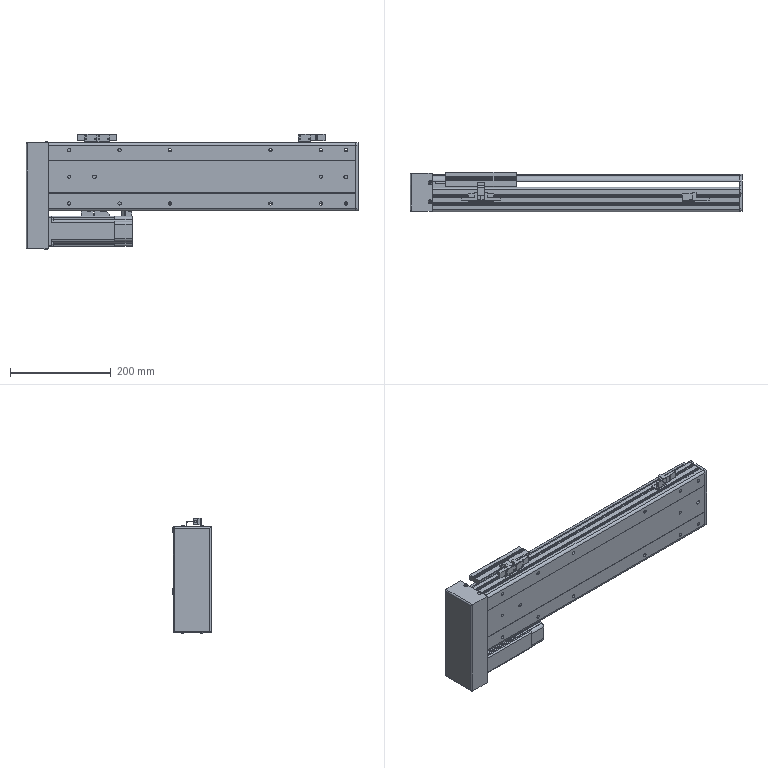Part | SolidWorks | 12 solids | 776 faces | box 660 x 78 x 229.35 mm | volume 4358113 mm3 | plane 404 | cylinder 314 | cone 50 | torus 8 | commonest cylinder face diameters 6 x37 2 x36 1 x30 6.647 x24 11 x24 2.5 x18